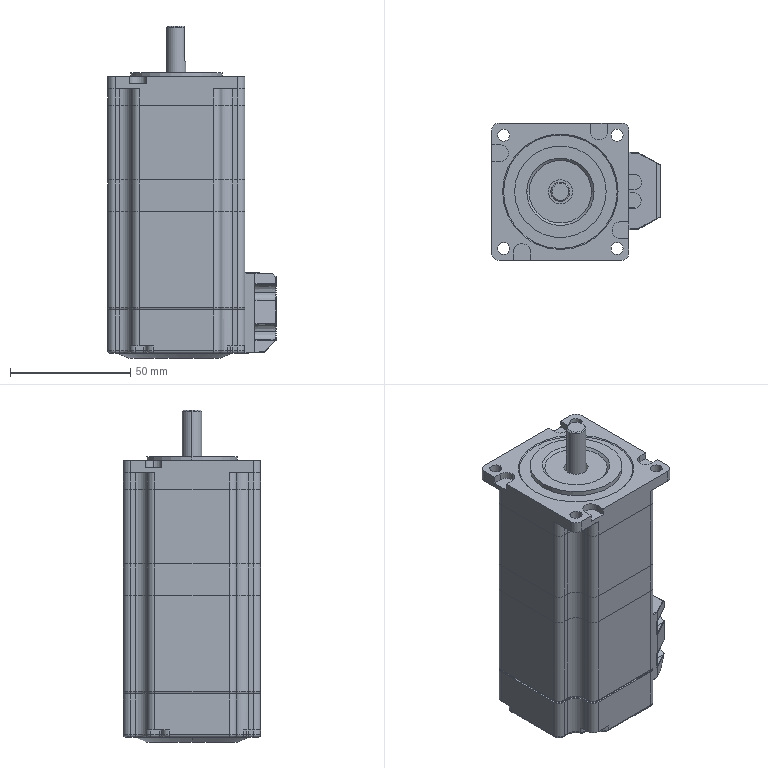Part | SolidWorks | 6 solids | 488 faces | box 70 x 57 x 138 mm | volume 311067 mm3 | cylinder 211 | plane 173 | torus 40 | spline 30 | sphere 18 | cone 16 | commonest cylinder face diameters 6 x48 0.4 x42 2 x32 10 x22 3 x8 3.1 x8